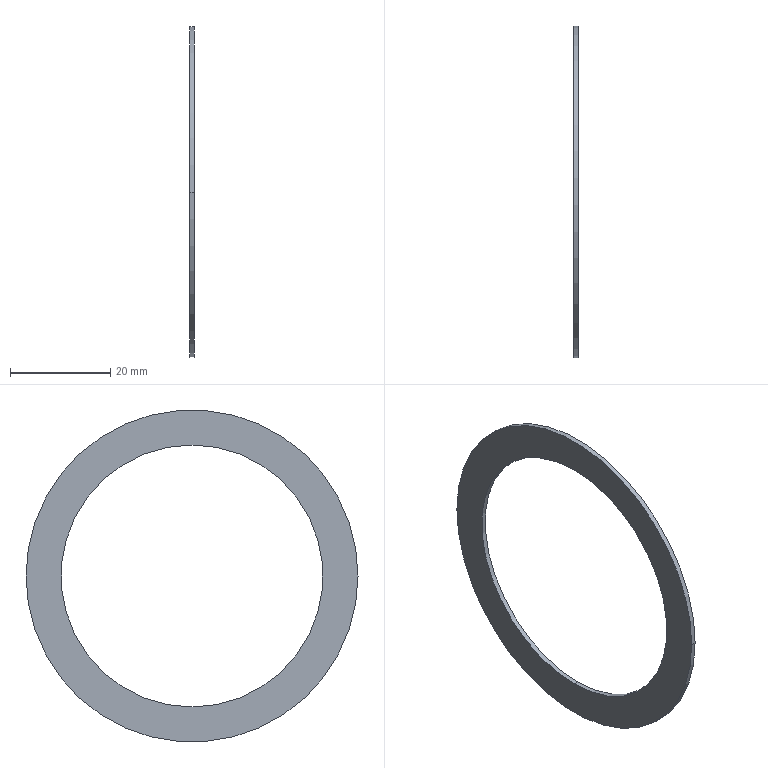Part | SolidWorks | features BaseBody 1 | 1 solid | 6 faces | box 0.99 x 66.3 x 66.3 mm | volume 1291 mm3 | cylinder 2 | spline 2 | plane 2 | commonest cylinder face diameters 66.3 x2
STEP:
#1=CARTESIAN_POINT('',(12.08,41.85,49.2));
#2=VERTEX_POINT('',#1);
#3=CARTESIAN_POINT('',(12.08,108.15,49.2));
#4=VERTEX_POINT('',#3);
#5=CARTESIAN_POINT('',(12.08,75.,49.2));
#6=DIRECTION('',(-1.,0.,0.));
#7=DIRECTION('',(0.,0.,1.));
#8=AXIS2_PLACEMENT_3D('',#5,#6,#7);
#9=CIRCLE('',#8,33.15);
#10=EDGE_CURVE('',#2,#4,#9,.T.);
#11=ORIENTED_EDGE('',*,*,#10,.T.);
#12=CARTESIAN_POINT('',(11.09,108.15,49.2));
#13=VERTEX_POINT('',#12);
#14=CARTESIAN_POINT('',(11.585,108.15,49.2));
#15=DIRECTION('',(-1.,0.,0.));
#16=VECTOR('',#15,1000.);
#17=LINE('',#14,#16);
#18=EDGE_CURVE('',#4,#13,#17,.T.);
#19=ORIENTED_EDGE('',*,*,#18,.T.);
#20=CARTESIAN_POINT('',(11.09,41.85,49.2));
#21=VERTEX_POINT('',#20);
#22=CARTESIAN_POINT('',(11.09,75.,49.2));
#23=DIRECTION('',(-1.,0.,0.));
#24=DIRECTION('',(0.,0.,1.));
#25=AXIS2_PLACEMENT_3D('',#22,#23,#24);
#26=CIRCLE('',#25,33.15);
#27=EDGE_CURVE('',#21,#13,#26,.T.);
#28=ORIENTED_EDGE('',*,*,#27,.F.);
#29=CARTESIAN_POINT('',(11.585,41.85,49.2));
#30=DIRECTION('',(-1.,0.,0.));
#31=VECTOR('',#30,1000.);
#32=LINE('',#29,#31);
#33=EDGE_CURVE('',#2,#21,#32,.T.);
#34=ORIENTED_EDGE('',*,*,#33,.F.);
#35=EDGE_LOOP('',(#11,#19,#28,#34));
#36=FACE_OUTER_BOUND('',#35,.T.);
#37=CARTESIAN_POINT('',(11.585,75.,49.2));
#38=DIRECTION('',(-1.,0.,0.));
#39=DIRECTION('',(0.,-1.,0.));
#40=AXIS2_PLACEMENT_3D('',#37,#38,#39);
#41=CYLINDRICAL_SURFACE('',#40,33.15);
#42=ADVANCED_FACE('',(#36),#41,.T.);
#43=CARTESIAN_POINT('',(12.08,75.,23.05));
#44=VERTEX_POINT('',#43);
#45=CARTESIAN_POINT('',(12.08,75.,75.35));
#46=VERTEX_POINT('',#45);
#47=CARTESIAN_POINT('',(12.08,75.,49.2));
#48=DIRECTION('',(-1.,0.,0.));
#49=DIRECTION('',(0.,0.,1.));
#50=AXIS2_PLACEMENT_3D('',#47,#48,#49);
#51=CIRCLE('',#50,26.15);
#52=EDGE_CURVE('',#44,#46,#51,.T.);
#53=ORIENTED_EDGE('',*,*,#52,.F.);
#54=CARTESIAN_POINT('',(11.09,75.,23.05));
#55=VERTEX_POINT('',#54);
#56=CARTESIAN_POINT('',(11.585,75.,23.05));
#57=DIRECTION('',(-1.,0.,0.));
#58=VECTOR('',#57,1000.);
#59=LINE('',#56,#58);
#60=EDGE_CURVE('',#44,#55,#59,.T.);
#61=ORIENTED_EDGE('',*,*,#60,.T.);
#62=CARTESIAN_POINT('',(11.09,75.,75.35));
#63=VERTEX_POINT('',#62);
#64=CARTESIAN_POINT('',(11.09,75.,49.2));
#65=DIRECTION('',(-1.,0.,0.));
#66=DIRECTION('',(0.,0.,1.));
#67=AXIS2_PLACEMENT_3D('',#64,#65,#66);
#68=CIRCLE('',#67,26.15);
#69=EDGE_CURVE('',#55,#63,#68,.T.);
#70=ORIENTED_EDGE('',*,*,#69,.T.);
#71=CARTESIAN_POINT('',(11.585,75.,75.35));
#72=DIRECTION('',(-1.,0.,0.));
#73=VECTOR('',#72,1000.);
#74=LINE('',#71,#73);
#75=EDGE_CURVE('',#46,#63,#74,.T.);
#76=ORIENTED_EDGE('',*,*,#75,.F.);
#77=EDGE_LOOP('',(#53,#61,#70,#76));
#78=FACE_OUTER_BOUND('',#77,.T.);
#79=CARTESIAN_POINT('',(12.08,75.,75.35));
#80=CARTESIAN_POINT('',(11.09,75.,75.35));
#81=CARTESIAN_POINT('',(12.08,22.7,75.35));
#82=CARTESIAN_POINT('',(11.09,22.7,75.35));
#83=CARTESIAN_POINT('',(12.08,22.7,23.05));
#84=CARTESIAN_POINT('',(11.09,22.7,23.05));
#85=CARTESIAN_POINT('',(12.08,75.,23.05));
#86=CARTESIAN_POINT('',(11.09,75.,23.05));
#87=(BOUNDED_SURFACE()B_SPLINE_SURFACE(3,1,((#79,#80),(#81,#82),(#83,#84),(#85,#86)),.UNSPECIFIED.,.F.,.F.,.F.)B_SPLINE_SURFACE_WITH_KNOTS((4,4),(2,2),(0.,1.),(0.,1.),.UNSPECIFIED.)GEOMETRIC_REPRESENTATION_ITEM()RATIONAL_B_SPLINE_SURFACE(((1.,1.),(0.3333,0.3333),(0.3333,0.3333),(1.,1.)))REPRESENTATION_ITEM('')SURFACE());
#88=ADVANCED_FACE('',(#78),#87,.T.);
#89=CARTESIAN_POINT('',(12.08,75.,49.2));
#90=DIRECTION('',(-1.,0.,0.));
#91=DIRECTION('',(0.,0.,1.));
#92=AXIS2_PLACEMENT_3D('',#89,#90,#91);
#93=CIRCLE('',#92,26.15);
#94=EDGE_CURVE('',#46,#44,#93,.T.);
#95=ORIENTED_EDGE('',*,*,#94,.T.);
#96=ORIENTED_EDGE('',*,*,#52,.T.);
#97=EDGE_LOOP('',(#95,#96));
#98=FACE_BOUND('',#97,.T.);
#99=ORIENTED_EDGE('',*,*,#10,.F.);
#100=CARTESIAN_POINT('',(12.08,75.,49.2));
#101=DIRECTION('',(-1.,0.,0.));
#102=DIRECTION('',(0.,0.,1.));
#103=AXIS2_PLACEMENT_3D('',#100,#101,#102);
#104=CIRCLE('',#103,33.15);
#105=EDGE_CURVE('',#4,#2,#104,.T.);
#106=ORIENTED_EDGE('',*,*,#105,.F.);
#107=EDGE_LOOP('',(#99,#106));
#108=FACE_OUTER_BOUND('',#107,.T.);
#109=CARTESIAN_POINT('',(12.08,75.,78.85));
#110=DIRECTION('',(1.,0.,0.));
#111=DIRECTION('',(0.,1.,0.));
#112=AXIS2_PLACEMENT_3D('',#109,#110,#111);
#113=PLANE('',#112);
#114=ADVANCED_FACE('',(#98,#108),#113,.T.);
#115=ORIENTED_EDGE('',*,*,#60,.F.);
#116=ORIENTED_EDGE('',*,*,#94,.F.);
#117=ORIENTED_EDGE('',*,*,#75,.T.);
#118=CARTESIAN_POINT('',(11.09,75.,49.2));
#119=DIRECTION('',(-1.,0.,0.));
#120=DIRECTION('',(0.,0.,1.));
#121=AXIS2_PLACEMENT_3D('',#118,#119,#120);
#122=CIRCLE('',#121,26.15);
#123=EDGE_CURVE('',#63,#55,#122,.T.);
#124=ORIENTED_EDGE('',*,*,#123,.T.);
#125=EDGE_LOOP('',(#115,#116,#117,#124));
#126=FACE_OUTER_BOUND('',#125,.T.);
#127=CARTESIAN_POINT('',(12.08,75.,23.05));
#128=CARTESIAN_POINT('',(11.09,75.,23.05));
#129=CARTESIAN_POINT('',(12.08,127.3,23.05));
#130=CARTESIAN_POINT('',(11.09,127.3,23.05));
#131=CARTESIAN_POINT('',(12.08,127.3,75.35));
#132=CARTESIAN_POINT('',(11.09,127.3,75.35));
#133=CARTESIAN_POINT('',(12.08,75.,75.35));
#134=CARTESIAN_POINT('',(11.09,75.,75.35));
#135=(BOUNDED_SURFACE()B_SPLINE_SURFACE(3,1,((#127,#128),(#129,#130),(#131,#132),(#133,#134)),.UNSPECIFIED.,.F.,.F.,.F.)B_SPLINE_SURFACE_WITH_KNOTS((4,4),(2,2),(0.,1.),(0.,1.),.UNSPECIFIED.)GEOMETRIC_REPRESENTATION_ITEM()RATIONAL_B_SPLINE_SURFACE(((1.,1.),(0.3333,0.3333),(0.3333,0.3333),(1.,1.)))REPRESENTATION_ITEM('')SURFACE());
#136=ADVANCED_FACE('',(#126),#135,.T.);
#137=ORIENTED_EDGE('',*,*,#27,.T.);
#138=CARTESIAN_POINT('',(11.09,75.,49.2));
#139=DIRECTION('',(-1.,0.,0.));
#140=DIRECTION('',(0.,0.,1.));
#141=AXIS2_PLACEMENT_3D('',#138,#139,#140);
#142=CIRCLE('',#141,33.15);
#143=EDGE_CURVE('',#13,#21,#142,.T.);
#144=ORIENTED_EDGE('',*,*,#143,.T.);
#145=EDGE_LOOP('',(#137,#144));
#146=FACE_OUTER_BOUND('',#145,.T.);
#147=ORIENTED_EDGE('',*,*,#123,.F.);
#148=ORIENTED_EDGE('',*,*,#69,.F.);
#149=EDGE_LOOP('',(#147,#148));
#150=FACE_BOUND('',#149,.T.);
#151=CARTESIAN_POINT('',(11.09,75.,78.85));
#152=DIRECTION('',(-1.,0.,0.));
#153=DIRECTION('',(0.,-1.,0.));
#154=AXIS2_PLACEMENT_3D('',#151,#152,#153);
#155=PLANE('',#154);
#156=ADVANCED_FACE('',(#146,#150),#155,.T.);
#157=ORIENTED_EDGE('',*,*,#18,.F.);
#158=ORIENTED_EDGE('',*,*,#105,.T.);
#159=ORIENTED_EDGE('',*,*,#33,.T.);
#160=ORIENTED_EDGE('',*,*,#143,.F.);
#161=EDGE_LOOP('',(#157,#158,#159,#160));
#162=FACE_OUTER_BOUND('',#161,.T.);
#163=CARTESIAN_POINT('',(11.585,75.,49.2));
#164=DIRECTION('',(-1.,0.,0.));
#165=DIRECTION('',(0.,-1.,0.));
#166=AXIS2_PLACEMENT_3D('',#163,#164,#165);
#167=CYLINDRICAL_SURFACE('',#166,33.15);
#168=ADVANCED_FACE('',(#162),#167,.T.);
#169=CLOSED_SHELL('',(#42,#88,#114,#136,#156,#168));
#170=MANIFOLD_SOLID_BREP('',#169);
#171=CARTESIAN_POINT('',(0.,0.,0.));
#172=DIRECTION('',(0.,0.,1.));
#173=DIRECTION('',(1.,0.,0.));
#174=AXIS2_PLACEMENT_3D('',#171,#172,#173);
#175=(LENGTH_UNIT()NAMED_UNIT(*)SI_UNIT(.MILLI.,.METRE.));
#176=UNCERTAINTY_MEASURE_WITH_UNIT(LENGTH_MEASURE(0.00001),#175,'','');
#177=(NAMED_UNIT(*)PLANE_ANGLE_UNIT()SI_UNIT($,.RADIAN.));
#178=(NAMED_UNIT(*)SI_UNIT($,.STERADIAN.)SOLID_ANGLE_UNIT());
#179=(GEOMETRIC_REPRESENTATION_CONTEXT(3)GLOBAL_UNCERTAINTY_ASSIGNED_CONTEXT((#176))GLOBAL_UNIT_ASSIGNED_CONTEXT((#175,#177,#178))REPRESENTATION_CONTEXT('',''));
#180=ADVANCED_BREP_SHAPE_REPRESENTATION('',(#170,#174),#179);